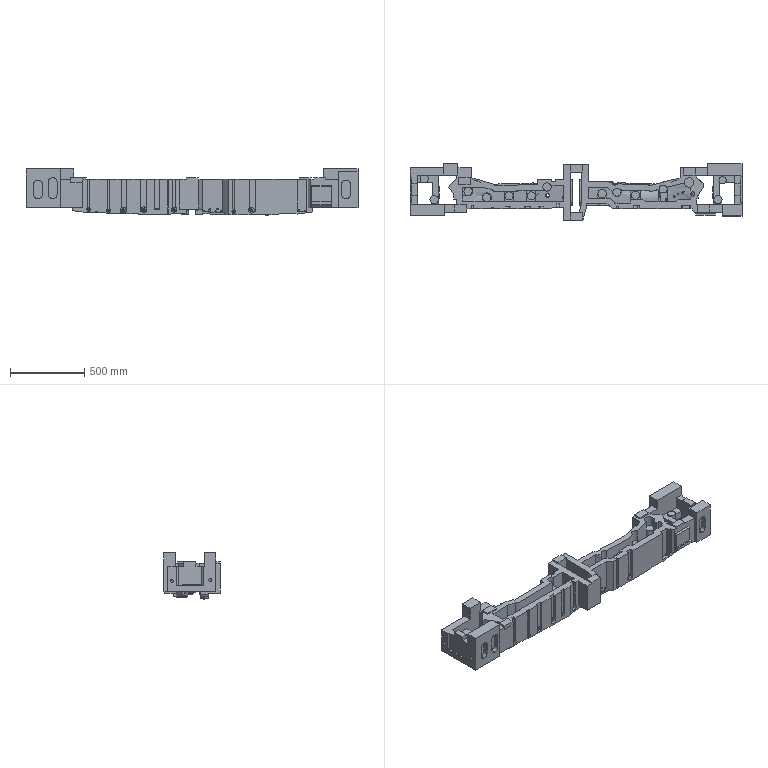Part | NX | features solid 2 | 1 solid | 1045 faces | box 2230 x 378.324 x 310.392 mm | volume 68483277 mm3 | plane 395 | spline 356 | cylinder 244 | sphere 18 | torus 16 | cone 16 | commonest cylinder face diameters 10 x46 20 x25 55 x18 50 x13 52 x12 11 x11